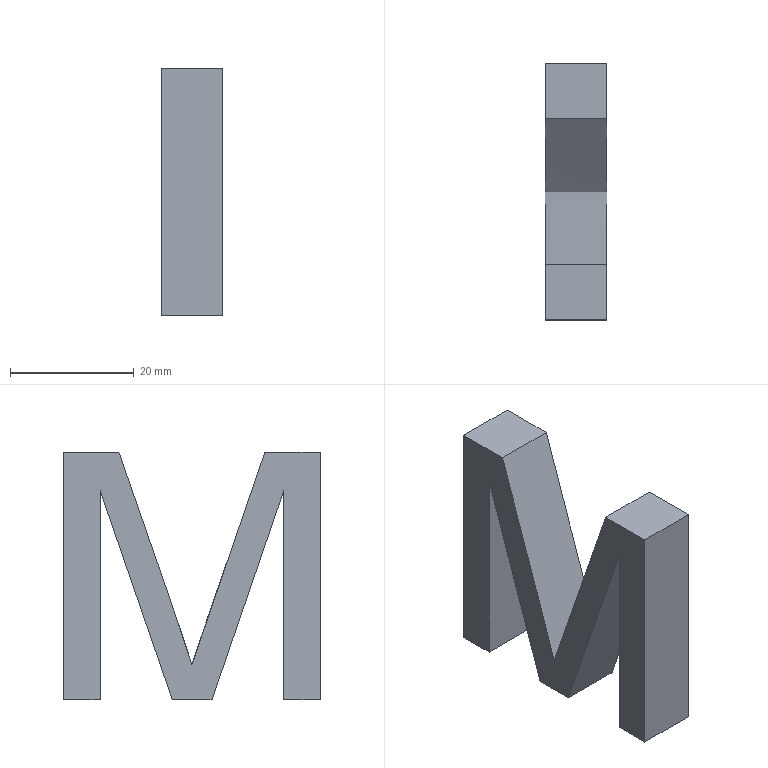Part | NX | features solid 2 | 1 solid | 15 faces | box 10 x 41.407 x 40 mm | volume 8614 mm3 | plane 13 | spline 2
STEP:
#1=CARTESIAN_POINT('',(2250.,-67.941,-590.));
#2=VERTEX_POINT('',#1);
#3=CARTESIAN_POINT('',(2250.,-73.8,-590.));
#4=VERTEX_POINT('',#3);
#5=CARTESIAN_POINT('',(2250.,-67.941,-590.));
#6=CARTESIAN_POINT('',(2250.,-69.894,-590.));
#7=CARTESIAN_POINT('',(2250.,-71.847,-590.));
#8=CARTESIAN_POINT('',(2250.,-73.8,-590.));
#9=B_SPLINE_CURVE_WITH_KNOTS('',3,(#5,#6,#7,#8),.UNSPECIFIED.,.F.,.F.,(4,4),(0.,0.01854),.PIECEWISE_BEZIER_KNOTS.);
#10=EDGE_CURVE('',#2,#4,#9,.T.);
#11=ORIENTED_EDGE('',*,*,#10,.F.);
#12=CARTESIAN_POINT('',(2260.,-67.941,-590.));
#13=VERTEX_POINT('',#12);
#14=CARTESIAN_POINT('',(2260.,-67.941,-590.));
#15=DIRECTION('',(-1.,0.,0.));
#16=VECTOR('',#15,1000.);
#17=LINE('',#14,#16);
#18=EDGE_CURVE('',#13,#2,#17,.T.);
#19=ORIENTED_EDGE('',*,*,#18,.F.);
#20=CARTESIAN_POINT('',(2260.,-73.8,-590.));
#21=VERTEX_POINT('',#20);
#22=CARTESIAN_POINT('',(2260.,-67.941,-590.));
#23=CARTESIAN_POINT('',(2260.,-69.894,-590.));
#24=CARTESIAN_POINT('',(2260.,-71.847,-590.));
#25=CARTESIAN_POINT('',(2260.,-73.8,-590.));
#26=B_SPLINE_CURVE_WITH_KNOTS('',3,(#22,#23,#24,#25),.UNSPECIFIED.,.F.,.F.,(4,4),(0.,0.01854),.PIECEWISE_BEZIER_KNOTS.);
#27=EDGE_CURVE('',#13,#21,#26,.T.);
#28=ORIENTED_EDGE('',*,*,#27,.T.);
#29=CARTESIAN_POINT('',(2260.,-73.8,-590.));
#30=DIRECTION('',(-1.,0.,0.));
#31=VECTOR('',#30,1000.);
#32=LINE('',#29,#31);
#33=EDGE_CURVE('',#21,#4,#32,.T.);
#34=ORIENTED_EDGE('',*,*,#33,.T.);
#35=EDGE_LOOP('',(#11,#19,#28,#34));
#36=FACE_BOUND('',#35,.T.);
#37=CARTESIAN_POINT('',(2260.,-67.941,-590.));
#38=DIRECTION('',(0.,0.,-1.));
#39=DIRECTION('',(-1.,0.,0.));
#40=AXIS2_PLACEMENT_3D('',#37,#38,#39);
#41=PLANE('',#40);
#42=ADVANCED_FACE('',(#36),#41,.T.);
#43=CARTESIAN_POINT('',(2250.,-73.8,-550.));
#44=VERTEX_POINT('',#43);
#45=CARTESIAN_POINT('',(2250.,-73.8,-590.));
#46=CARTESIAN_POINT('',(2250.,-73.8,-576.667));
#47=CARTESIAN_POINT('',(2250.,-73.8,-563.333));
#48=CARTESIAN_POINT('',(2250.,-73.8,-550.));
#49=B_SPLINE_CURVE_WITH_KNOTS('',3,(#45,#46,#47,#48),.UNSPECIFIED.,.F.,.F.,(4,4),(0.01854,0.1451),.PIECEWISE_BEZIER_KNOTS.);
#50=EDGE_CURVE('',#4,#44,#49,.T.);
#51=ORIENTED_EDGE('',*,*,#50,.F.);
#52=ORIENTED_EDGE('',*,*,#33,.F.);
#53=CARTESIAN_POINT('',(2260.,-73.8,-550.));
#54=VERTEX_POINT('',#53);
#55=CARTESIAN_POINT('',(2260.,-73.8,-590.));
#56=CARTESIAN_POINT('',(2260.,-73.8,-576.667));
#57=CARTESIAN_POINT('',(2260.,-73.8,-563.333));
#58=CARTESIAN_POINT('',(2260.,-73.8,-550.));
#59=B_SPLINE_CURVE_WITH_KNOTS('',3,(#55,#56,#57,#58),.UNSPECIFIED.,.F.,.F.,(4,4),(0.01854,0.1451),.PIECEWISE_BEZIER_KNOTS.);
#60=EDGE_CURVE('',#21,#54,#59,.T.);
#61=ORIENTED_EDGE('',*,*,#60,.T.);
#62=CARTESIAN_POINT('',(2260.,-73.8,-550.));
#63=DIRECTION('',(-1.,0.,0.));
#64=VECTOR('',#63,1000.);
#65=LINE('',#62,#64);
#66=EDGE_CURVE('',#54,#44,#65,.T.);
#67=ORIENTED_EDGE('',*,*,#66,.T.);
#68=EDGE_LOOP('',(#51,#52,#61,#67));
#69=FACE_BOUND('',#68,.T.);
#70=CARTESIAN_POINT('',(2260.,-73.8,-590.));
#71=DIRECTION('',(0.,-1.,0.));
#72=DIRECTION('',(1.,0.,0.));
#73=AXIS2_PLACEMENT_3D('',#70,#71,#72);
#74=PLANE('',#73);
#75=ADVANCED_FACE('',(#69),#74,.T.);
#76=CARTESIAN_POINT('',(2250.,-64.852,-550.));
#77=VERTEX_POINT('',#76);
#78=CARTESIAN_POINT('',(2250.,-73.8,-550.));
#79=CARTESIAN_POINT('',(2250.,-70.817,-550.));
#80=CARTESIAN_POINT('',(2250.,-67.834,-550.));
#81=CARTESIAN_POINT('',(2250.,-64.852,-550.));
#82=B_SPLINE_CURVE_WITH_KNOTS('',3,(#78,#79,#80,#81),.UNSPECIFIED.,.F.,.F.,(4,4),(0.1451,0.1734),.PIECEWISE_BEZIER_KNOTS.);
#83=EDGE_CURVE('',#44,#77,#82,.T.);
#84=ORIENTED_EDGE('',*,*,#83,.F.);
#85=ORIENTED_EDGE('',*,*,#66,.F.);
#86=CARTESIAN_POINT('',(2260.,-64.852,-550.));
#87=VERTEX_POINT('',#86);
#88=CARTESIAN_POINT('',(2260.,-73.8,-550.));
#89=CARTESIAN_POINT('',(2260.,-70.817,-550.));
#90=CARTESIAN_POINT('',(2260.,-67.834,-550.));
#91=CARTESIAN_POINT('',(2260.,-64.852,-550.));
#92=B_SPLINE_CURVE_WITH_KNOTS('',3,(#88,#89,#90,#91),.UNSPECIFIED.,.F.,.F.,(4,4),(0.1451,0.1734),.PIECEWISE_BEZIER_KNOTS.);
#93=EDGE_CURVE('',#54,#87,#92,.T.);
#94=ORIENTED_EDGE('',*,*,#93,.T.);
#95=CARTESIAN_POINT('',(2260.,-64.852,-550.));
#96=DIRECTION('',(-1.,0.,0.));
#97=VECTOR('',#96,1000.);
#98=LINE('',#95,#97);
#99=EDGE_CURVE('',#87,#77,#98,.T.);
#100=ORIENTED_EDGE('',*,*,#99,.T.);
#101=EDGE_LOOP('',(#84,#85,#94,#100));
#102=FACE_BOUND('',#101,.T.);
#103=CARTESIAN_POINT('',(2260.,-73.8,-550.));
#104=DIRECTION('',(0.,0.,1.));
#105=DIRECTION('',(1.,0.,0.));
#106=AXIS2_PLACEMENT_3D('',#103,#104,#105);
#107=PLANE('',#106);
#108=ADVANCED_FACE('',(#102),#107,.T.);
#109=CARTESIAN_POINT('',(2250.,-53.089,-584.279));
#110=VERTEX_POINT('',#109);
#111=CARTESIAN_POINT('',(2250.,-64.852,-550.));
#112=CARTESIAN_POINT('',(2250.,-61.593,-559.453));
#113=CARTESIAN_POINT('',(2250.,-58.335,-568.906));
#114=CARTESIAN_POINT('',(2250.,-54.16,-581.021));
#115=CARTESIAN_POINT('',(2250.,-53.502,-582.994));
#116=CARTESIAN_POINT('',(2250.,-53.089,-584.279));
#117=B_SPLINE_CURVE_WITH_KNOTS('',3,(#111,#112,#113,#114,#115,#116),.UNSPECIFIED.,.F.,.F.,(4,2,4),(0.1734,0.2684,0.2951),.UNSPECIFIED.);
#118=EDGE_CURVE('',#77,#110,#117,.T.);
#119=ORIENTED_EDGE('',*,*,#118,.F.);
#120=ORIENTED_EDGE('',*,*,#99,.F.);
#121=CARTESIAN_POINT('',(2260.,-53.089,-584.279));
#122=VERTEX_POINT('',#121);
#123=CARTESIAN_POINT('',(2260.,-64.852,-550.));
#124=CARTESIAN_POINT('',(2260.,-61.593,-559.453));
#125=CARTESIAN_POINT('',(2260.,-58.335,-568.906));
#126=CARTESIAN_POINT('',(2260.,-54.16,-581.021));
#127=CARTESIAN_POINT('',(2260.,-53.502,-582.994));
#128=CARTESIAN_POINT('',(2260.,-53.089,-584.279));
#129=B_SPLINE_CURVE_WITH_KNOTS('',3,(#123,#124,#125,#126,#127,#128),.UNSPECIFIED.,.F.,.F.,(4,2,4),(0.1734,0.2684,0.2951),.UNSPECIFIED.);
#130=EDGE_CURVE('',#87,#122,#129,.T.);
#131=ORIENTED_EDGE('',*,*,#130,.T.);
#132=CARTESIAN_POINT('',(2260.,-53.089,-584.279));
#133=DIRECTION('',(-1.,0.,0.));
#134=VECTOR('',#133,1000.);
#135=LINE('',#132,#134);
#136=EDGE_CURVE('',#122,#110,#135,.T.);
#137=ORIENTED_EDGE('',*,*,#136,.T.);
#138=EDGE_LOOP('',(#119,#120,#131,#137));
#139=FACE_BOUND('',#138,.T.);
#140=CARTESIAN_POINT('',(2260.,-64.852,-550.));
#141=CARTESIAN_POINT('',(2250.,-64.852,-550.));
#142=CARTESIAN_POINT('',(2260.,-63.808,-553.029));
#143=CARTESIAN_POINT('',(2250.,-63.808,-553.029));
#144=CARTESIAN_POINT('',(2260.,-61.72,-559.087));
#145=CARTESIAN_POINT('',(2250.,-61.72,-559.087));
#146=CARTESIAN_POINT('',(2260.,-59.111,-566.656));
#147=CARTESIAN_POINT('',(2250.,-59.111,-566.656));
#148=CARTESIAN_POINT('',(2260.,-57.021,-572.719));
#149=CARTESIAN_POINT('',(2250.,-57.021,-572.719));
#150=CARTESIAN_POINT('',(2260.,-55.721,-576.492));
#151=CARTESIAN_POINT('',(2250.,-55.721,-576.492));
#152=CARTESIAN_POINT('',(2260.,-54.668,-579.546));
#153=CARTESIAN_POINT('',(2250.,-54.668,-579.546));
#154=CARTESIAN_POINT('',(2260.,-53.796,-582.114));
#155=CARTESIAN_POINT('',(2250.,-53.796,-582.114));
#156=CARTESIAN_POINT('',(2260.,-53.324,-583.548));
#157=CARTESIAN_POINT('',(2250.,-53.324,-583.548));
#158=CARTESIAN_POINT('',(2260.,-53.089,-584.279));
#159=CARTESIAN_POINT('',(2250.,-53.089,-584.279));
#160=B_SPLINE_SURFACE_WITH_KNOTS('',3,1,((#140,#141),(#142,#143),(#144,#145),(#146,#147),(#148,#149),(#150,#151),(#152,#153),(#154,#155),(#156,#157),(#158,#159)),.SURF_OF_LINEAR_EXTRUSION.,.F.,.F.,.F.,(4,1,1,1,1,1,1,4),(2,2),(0.1734,0.2039,0.2343,0.2495,0.2647,0.2723,0.2799,0.2951),(0.,1.),.UNSPECIFIED.);
#161=ADVANCED_FACE('',(#139),#160,.T.);
#162=CARTESIAN_POINT('',(2250.,-41.295,-550.));
#163=VERTEX_POINT('',#162);
#164=CARTESIAN_POINT('',(2250.,-53.089,-584.279));
#165=CARTESIAN_POINT('',(2250.,-52.615,-582.841));
#166=CARTESIAN_POINT('',(2250.,-51.911,-580.715));
#167=CARTESIAN_POINT('',(2250.,-47.793,-568.558));
#168=CARTESIAN_POINT('',(2250.,-44.513,-559.29));
#169=CARTESIAN_POINT('',(2250.,-41.295,-550.));
#170=B_SPLINE_CURVE_WITH_KNOTS('',3,(#164,#165,#166,#167,#168,#169),.UNSPECIFIED.,.F.,.F.,(4,2,4),(0.2951,0.317,0.3887),.UNSPECIFIED.);
#171=EDGE_CURVE('',#110,#163,#170,.T.);
#172=ORIENTED_EDGE('',*,*,#171,.F.);
#173=ORIENTED_EDGE('',*,*,#136,.F.);
#174=CARTESIAN_POINT('',(2260.,-41.295,-550.));
#175=VERTEX_POINT('',#174);
#176=CARTESIAN_POINT('',(2260.,-53.089,-584.279));
#177=CARTESIAN_POINT('',(2260.,-52.615,-582.841));
#178=CARTESIAN_POINT('',(2260.,-51.911,-580.715));
#179=CARTESIAN_POINT('',(2260.,-47.793,-568.558));
#180=CARTESIAN_POINT('',(2260.,-44.513,-559.29));
#181=CARTESIAN_POINT('',(2260.,-41.295,-550.));
#182=B_SPLINE_CURVE_WITH_KNOTS('',3,(#176,#177,#178,#179,#180,#181),.UNSPECIFIED.,.F.,.F.,(4,2,4),(0.2951,0.317,0.3887),.UNSPECIFIED.);
#183=EDGE_CURVE('',#122,#175,#182,.T.);
#184=ORIENTED_EDGE('',*,*,#183,.T.);
#185=CARTESIAN_POINT('',(2260.,-41.295,-550.));
#186=DIRECTION('',(-1.,0.,0.));
#187=VECTOR('',#186,1000.);
#188=LINE('',#185,#187);
#189=EDGE_CURVE('',#175,#163,#188,.T.);
#190=ORIENTED_EDGE('',*,*,#189,.T.);
#191=EDGE_LOOP('',(#172,#173,#184,#190));
#192=FACE_BOUND('',#191,.T.);
#193=CARTESIAN_POINT('',(2260.,-53.089,-584.279));
#194=CARTESIAN_POINT('',(2250.,-53.089,-584.279));
#195=CARTESIAN_POINT('',(2260.,-52.835,-583.511));
#196=CARTESIAN_POINT('',(2250.,-52.835,-583.511));
#197=CARTESIAN_POINT('',(2260.,-52.355,-582.059));
#198=CARTESIAN_POINT('',(2250.,-52.355,-582.059));
#199=CARTESIAN_POINT('',(2260.,-51.513,-579.543));
#200=CARTESIAN_POINT('',(2250.,-51.513,-579.543));
#201=CARTESIAN_POINT('',(2260.,-50.499,-576.542));
#202=CARTESIAN_POINT('',(2250.,-50.499,-576.542));
#203=CARTESIAN_POINT('',(2260.,-49.195,-572.727));
#204=CARTESIAN_POINT('',(2250.,-49.195,-572.727));
#205=CARTESIAN_POINT('',(2260.,-47.103,-566.669));
#206=CARTESIAN_POINT('',(2250.,-47.103,-566.669));
#207=CARTESIAN_POINT('',(2260.,-44.459,-559.091));
#208=CARTESIAN_POINT('',(2250.,-44.459,-559.091));
#209=CARTESIAN_POINT('',(2260.,-42.345,-553.032));
#210=CARTESIAN_POINT('',(2250.,-42.345,-553.032));
#211=CARTESIAN_POINT('',(2260.,-41.295,-550.));
#212=CARTESIAN_POINT('',(2250.,-41.295,-550.));
#213=B_SPLINE_SURFACE_WITH_KNOTS('',3,1,((#193,#194),(#195,#196),(#197,#198),(#199,#200),(#201,#202),(#203,#204),(#205,#206),(#207,#208),(#209,#210),(#211,#212)),.SURF_OF_LINEAR_EXTRUSION.,.F.,.F.,.F.,(4,1,1,1,1,1,1,4),(2,2),(0.2951,0.3068,0.3126,0.3185,0.3302,0.3419,0.3653,0.3887),(0.,1.),.UNSPECIFIED.);
#214=ADVANCED_FACE('',(#192),#213,.T.);
#215=CARTESIAN_POINT('',(2250.,-32.393,-550.));
#216=VERTEX_POINT('',#215);
#217=CARTESIAN_POINT('',(2250.,-41.295,-550.));
#218=CARTESIAN_POINT('',(2250.,-38.328,-550.));
#219=CARTESIAN_POINT('',(2250.,-35.36,-550.));
#220=CARTESIAN_POINT('',(2250.,-32.393,-550.));
#221=B_SPLINE_CURVE_WITH_KNOTS('',3,(#217,#218,#219,#220),.UNSPECIFIED.,.F.,.F.,(4,4),(0.3887,0.4159),.PIECEWISE_BEZIER_KNOTS.);
#222=EDGE_CURVE('',#163,#216,#221,.T.);
#223=ORIENTED_EDGE('',*,*,#222,.F.);
#224=ORIENTED_EDGE('',*,*,#189,.F.);
#225=CARTESIAN_POINT('',(2260.,-32.393,-550.));
#226=VERTEX_POINT('',#225);
#227=CARTESIAN_POINT('',(2260.,-41.295,-550.));
#228=CARTESIAN_POINT('',(2260.,-38.328,-550.));
#229=CARTESIAN_POINT('',(2260.,-35.36,-550.));
#230=CARTESIAN_POINT('',(2260.,-32.393,-550.));
#231=B_SPLINE_CURVE_WITH_KNOTS('',3,(#227,#228,#229,#230),.UNSPECIFIED.,.F.,.F.,(4,4),(0.3887,0.4159),.PIECEWISE_BEZIER_KNOTS.);
#232=EDGE_CURVE('',#175,#226,#231,.T.);
#233=ORIENTED_EDGE('',*,*,#232,.T.);
#234=CARTESIAN_POINT('',(2260.,-32.393,-550.));
#235=DIRECTION('',(-1.,0.,0.));
#236=VECTOR('',#235,1000.);
#237=LINE('',#234,#236);
#238=EDGE_CURVE('',#226,#216,#237,.T.);
#239=ORIENTED_EDGE('',*,*,#238,.T.);
#240=EDGE_LOOP('',(#223,#224,#233,#239));
#241=FACE_BOUND('',#240,.T.);
#242=CARTESIAN_POINT('',(2260.,-41.295,-550.));
#243=DIRECTION('',(0.,0.,1.));
#244=DIRECTION('',(1.,0.,0.));
#245=AXIS2_PLACEMENT_3D('',#242,#243,#244);
#246=PLANE('',#245);
#247=ADVANCED_FACE('',(#241),#246,.T.);
#248=CARTESIAN_POINT('',(2250.,-32.393,-590.));
#249=VERTEX_POINT('',#248);
#250=CARTESIAN_POINT('',(2250.,-32.393,-550.));
#251=CARTESIAN_POINT('',(2250.,-32.393,-563.333));
#252=CARTESIAN_POINT('',(2250.,-32.393,-576.667));
#253=CARTESIAN_POINT('',(2250.,-32.393,-590.));
#254=B_SPLINE_CURVE_WITH_KNOTS('',3,(#250,#251,#252,#253),.UNSPECIFIED.,.F.,.F.,(4,4),(0.4159,0.538),.PIECEWISE_BEZIER_KNOTS.);
#255=EDGE_CURVE('',#216,#249,#254,.T.);
#256=ORIENTED_EDGE('',*,*,#255,.F.);
#257=ORIENTED_EDGE('',*,*,#238,.F.);
#258=CARTESIAN_POINT('',(2260.,-32.393,-590.));
#259=VERTEX_POINT('',#258);
#260=CARTESIAN_POINT('',(2260.,-32.393,-550.));
#261=CARTESIAN_POINT('',(2260.,-32.393,-563.333));
#262=CARTESIAN_POINT('',(2260.,-32.393,-576.667));
#263=CARTESIAN_POINT('',(2260.,-32.393,-590.));
#264=B_SPLINE_CURVE_WITH_KNOTS('',3,(#260,#261,#262,#263),.UNSPECIFIED.,.F.,.F.,(4,4),(0.4159,0.538),.PIECEWISE_BEZIER_KNOTS.);
#265=EDGE_CURVE('',#226,#259,#264,.T.);
#266=ORIENTED_EDGE('',*,*,#265,.T.);
#267=CARTESIAN_POINT('',(2260.,-32.393,-590.));
#268=DIRECTION('',(-1.,0.,0.));
#269=VECTOR('',#268,1000.);
#270=LINE('',#267,#269);
#271=EDGE_CURVE('',#259,#249,#270,.T.);
#272=ORIENTED_EDGE('',*,*,#271,.T.);
#273=EDGE_LOOP('',(#256,#257,#266,#272));
#274=FACE_BOUND('',#273,.T.);
#275=CARTESIAN_POINT('',(2260.,-32.393,-550.));
#276=DIRECTION('',(0.,1.,0.));
#277=DIRECTION('',(-1.,0.,0.));
#278=AXIS2_PLACEMENT_3D('',#275,#276,#277);
#279=PLANE('',#278);
#280=ADVANCED_FACE('',(#274),#279,.T.);
#281=CARTESIAN_POINT('',(2250.,-38.236,-590.));
#282=VERTEX_POINT('',#281);
#283=CARTESIAN_POINT('',(2250.,-32.393,-590.));
#284=CARTESIAN_POINT('',(2250.,-34.34,-590.));
#285=CARTESIAN_POINT('',(2250.,-36.288,-590.));
#286=CARTESIAN_POINT('',(2250.,-38.236,-590.));
#287=B_SPLINE_CURVE_WITH_KNOTS('',3,(#283,#284,#285,#286),.UNSPECIFIED.,.F.,.F.,(4,4),(0.538,0.5558),.PIECEWISE_BEZIER_KNOTS.);
#288=EDGE_CURVE('',#249,#282,#287,.T.);
#289=ORIENTED_EDGE('',*,*,#288,.F.);
#290=ORIENTED_EDGE('',*,*,#271,.F.);
#291=CARTESIAN_POINT('',(2260.,-38.236,-590.));
#292=VERTEX_POINT('',#291);
#293=CARTESIAN_POINT('',(2260.,-32.393,-590.));
#294=CARTESIAN_POINT('',(2260.,-34.34,-590.));
#295=CARTESIAN_POINT('',(2260.,-36.288,-590.));
#296=CARTESIAN_POINT('',(2260.,-38.236,-590.));
#297=B_SPLINE_CURVE_WITH_KNOTS('',3,(#293,#294,#295,#296),.UNSPECIFIED.,.F.,.F.,(4,4),(0.538,0.5558),.PIECEWISE_BEZIER_KNOTS.);
#298=EDGE_CURVE('',#259,#292,#297,.T.);
#299=ORIENTED_EDGE('',*,*,#298,.T.);
#300=CARTESIAN_POINT('',(2260.,-38.236,-590.));
#301=DIRECTION('',(-1.,0.,0.));
#302=VECTOR('',#301,1000.);
#303=LINE('',#300,#302);
#304=EDGE_CURVE('',#292,#282,#303,.T.);
#305=ORIENTED_EDGE('',*,*,#304,.T.);
#306=EDGE_LOOP('',(#289,#290,#299,#305));
#307=FACE_BOUND('',#306,.T.);
#308=CARTESIAN_POINT('',(2260.,-32.393,-590.));
#309=DIRECTION('',(0.,0.,-1.));
#310=DIRECTION('',(-1.,0.,0.));
#311=AXIS2_PLACEMENT_3D('',#308,#309,#310);
#312=PLANE('',#311);
#313=ADVANCED_FACE('',(#307),#312,.T.);
#314=CARTESIAN_POINT('',(2250.,-38.236,-556.21));
#315=VERTEX_POINT('',#314);
#316=CARTESIAN_POINT('',(2250.,-38.236,-590.));
#317=CARTESIAN_POINT('',(2250.,-38.236,-578.737));
#318=CARTESIAN_POINT('',(2250.,-38.236,-567.474));
#319=CARTESIAN_POINT('',(2250.,-38.236,-556.21));
#320=B_SPLINE_CURVE_WITH_KNOTS('',3,(#316,#317,#318,#319),.UNSPECIFIED.,.F.,.F.,(4,4),(0.5558,0.659),.PIECEWISE_BEZIER_KNOTS.);
#321=EDGE_CURVE('',#282,#315,#320,.T.);
#322=ORIENTED_EDGE('',*,*,#321,.F.);
#323=ORIENTED_EDGE('',*,*,#304,.F.);
#324=CARTESIAN_POINT('',(2260.,-38.236,-556.21));
#325=VERTEX_POINT('',#324);
#326=CARTESIAN_POINT('',(2260.,-38.236,-590.));
#327=CARTESIAN_POINT('',(2260.,-38.236,-578.737));
#328=CARTESIAN_POINT('',(2260.,-38.236,-567.474));
#329=CARTESIAN_POINT('',(2260.,-38.236,-556.21));
#330=B_SPLINE_CURVE_WITH_KNOTS('',3,(#326,#327,#328,#329),.UNSPECIFIED.,.F.,.F.,(4,4),(0.5558,0.659),.PIECEWISE_BEZIER_KNOTS.);
#331=EDGE_CURVE('',#292,#325,#330,.T.);
#332=ORIENTED_EDGE('',*,*,#331,.T.);
#333=CARTESIAN_POINT('',(2260.,-38.236,-556.21));
#334=DIRECTION('',(-1.,0.,0.));
#335=VECTOR('',#334,1000.);
#336=LINE('',#333,#335);
#337=EDGE_CURVE('',#325,#315,#336,.T.);
#338=ORIENTED_EDGE('',*,*,#337,.T.);
#339=EDGE_LOOP('',(#322,#323,#332,#338));
#340=FACE_BOUND('',#339,.T.);
#341=CARTESIAN_POINT('',(2260.,-38.236,-590.));
#342=DIRECTION('',(0.,-1.,0.));
#343=DIRECTION('',(1.,0.,0.));
#344=AXIS2_PLACEMENT_3D('',#341,#342,#343);
#345=PLANE('',#344);
#346=ADVANCED_FACE('',(#340),#345,.T.);
#347=CARTESIAN_POINT('',(2250.,-49.907,-590.));
#348=VERTEX_POINT('',#347);
#349=CARTESIAN_POINT('',(2250.,-38.236,-556.21));
#350=CARTESIAN_POINT('',(2250.,-42.126,-567.474));
#351=CARTESIAN_POINT('',(2250.,-46.017,-578.737));
#352=CARTESIAN_POINT('',(2250.,-49.907,-590.));
#353=B_SPLINE_CURVE_WITH_KNOTS('',3,(#349,#350,#351,#352),.UNSPECIFIED.,.F.,.F.,(4,4),(0.659,0.7681),.PIECEWISE_BEZIER_KNOTS.);
#354=EDGE_CURVE('',#315,#348,#353,.T.);
#355=ORIENTED_EDGE('',*,*,#354,.F.);
#356=ORIENTED_EDGE('',*,*,#337,.F.);
#357=CARTESIAN_POINT('',(2260.,-49.907,-590.));
#358=VERTEX_POINT('',#357);
#359=CARTESIAN_POINT('',(2260.,-38.236,-556.21));
#360=CARTESIAN_POINT('',(2260.,-42.126,-567.474));
#361=CARTESIAN_POINT('',(2260.,-46.017,-578.737));
#362=CARTESIAN_POINT('',(2260.,-49.907,-590.));
#363=B_SPLINE_CURVE_WITH_KNOTS('',3,(#359,#360,#361,#362),.UNSPECIFIED.,.F.,.F.,(4,4),(0.659,0.7681),.PIECEWISE_BEZIER_KNOTS.);
#364=EDGE_CURVE('',#325,#358,#363,.T.);
#365=ORIENTED_EDGE('',*,*,#364,.T.);
#366=CARTESIAN_POINT('',(2260.,-49.907,-590.));
#367=DIRECTION('',(-1.,0.,0.));
#368=VECTOR('',#367,1000.);
#369=LINE('',#366,#368);
#370=EDGE_CURVE('',#358,#348,#369,.T.);
#371=ORIENTED_EDGE('',*,*,#370,.T.);
#372=EDGE_LOOP('',(#355,#356,#365,#371));
#373=FACE_BOUND('',#372,.T.);
#374=CARTESIAN_POINT('',(2260.,-38.236,-556.21));
#375=DIRECTION('',(0.,0.9452,-0.3265));
#376=DIRECTION('',(0.,0.3265,0.9452));
#377=AXIS2_PLACEMENT_3D('',#374,#375,#376);
#378=PLANE('',#377);
#379=ADVANCED_FACE('',(#373),#378,.T.);
#380=CARTESIAN_POINT('',(2250.,-56.332,-590.));
#381=VERTEX_POINT('',#380);
#382=CARTESIAN_POINT('',(2250.,-49.907,-590.));
#383=CARTESIAN_POINT('',(2250.,-52.049,-590.));
#384=CARTESIAN_POINT('',(2250.,-54.19,-590.));
#385=CARTESIAN_POINT('',(2250.,-56.332,-590.));
#386=B_SPLINE_CURVE_WITH_KNOTS('',3,(#382,#383,#384,#385),.UNSPECIFIED.,.F.,.F.,(4,4),(0.7681,0.7877),.PIECEWISE_BEZIER_KNOTS.);
#387=EDGE_CURVE('',#348,#381,#386,.T.);
#388=ORIENTED_EDGE('',*,*,#387,.F.);
#389=ORIENTED_EDGE('',*,*,#370,.F.);
#390=CARTESIAN_POINT('',(2260.,-56.332,-590.));
#391=VERTEX_POINT('',#390);
#392=CARTESIAN_POINT('',(2260.,-49.907,-590.));
#393=CARTESIAN_POINT('',(2260.,-52.049,-590.));
#394=CARTESIAN_POINT('',(2260.,-54.19,-590.));
#395=CARTESIAN_POINT('',(2260.,-56.332,-590.));
#396=B_SPLINE_CURVE_WITH_KNOTS('',3,(#392,#393,#394,#395),.UNSPECIFIED.,.F.,.F.,(4,4),(0.7681,0.7877),.PIECEWISE_BEZIER_KNOTS.);
#397=EDGE_CURVE('',#358,#391,#396,.T.);
#398=ORIENTED_EDGE('',*,*,#397,.T.);
#399=CARTESIAN_POINT('',(2260.,-56.332,-590.));
#400=DIRECTION('',(-1.,0.,0.));
#401=VECTOR('',#400,1000.);
#402=LINE('',#399,#401);
#403=EDGE_CURVE('',#391,#381,#402,.T.);
#404=ORIENTED_EDGE('',*,*,#403,.T.);
#405=EDGE_LOOP('',(#388,#389,#398,#404));
#406=FACE_BOUND('',#405,.T.);
#407=CARTESIAN_POINT('',(2260.,-49.907,-590.));
#408=DIRECTION('',(0.,0.,-1.));
#409=DIRECTION('',(-1.,0.,0.));
#410=AXIS2_PLACEMENT_3D('',#407,#408,#409);
#411=PLANE('',#410);
#412=ADVANCED_FACE('',(#406),#411,.T.);
#413=CARTESIAN_POINT('',(2250.,-67.941,-556.21));
#414=VERTEX_POINT('',#413);
#415=CARTESIAN_POINT('',(2250.,-56.332,-590.));
#416=CARTESIAN_POINT('',(2250.,-60.202,-578.737));
#417=CARTESIAN_POINT('',(2250.,-64.072,-567.474));
#418=CARTESIAN_POINT('',(2250.,-67.941,-556.21));
#419=B_SPLINE_CURVE_WITH_KNOTS('',3,(#415,#416,#417,#418),.UNSPECIFIED.,.F.,.F.,(4,4),(0.7877,0.8968),.PIECEWISE_BEZIER_KNOTS.);
#420=EDGE_CURVE('',#381,#414,#419,.T.);
#421=ORIENTED_EDGE('',*,*,#420,.F.);
#422=ORIENTED_EDGE('',*,*,#403,.F.);
#423=CARTESIAN_POINT('',(2260.,-67.941,-556.21));
#424=VERTEX_POINT('',#423);
#425=CARTESIAN_POINT('',(2260.,-56.332,-590.));
#426=CARTESIAN_POINT('',(2260.,-60.202,-578.737));
#427=CARTESIAN_POINT('',(2260.,-64.072,-567.474));
#428=CARTESIAN_POINT('',(2260.,-67.941,-556.21));
#429=B_SPLINE_CURVE_WITH_KNOTS('',3,(#425,#426,#427,#428),.UNSPECIFIED.,.F.,.F.,(4,4),(0.7877,0.8968),.PIECEWISE_BEZIER_KNOTS.);
#430=EDGE_CURVE('',#391,#424,#429,.T.);
#431=ORIENTED_EDGE('',*,*,#430,.T.);
#432=CARTESIAN_POINT('',(2260.,-67.941,-556.21));
#433=DIRECTION('',(-1.,0.,0.));
#434=VECTOR('',#433,1000.);
#435=LINE('',#432,#434);
#436=EDGE_CURVE('',#424,#414,#435,.T.);
#437=ORIENTED_EDGE('',*,*,#436,.T.);
#438=EDGE_LOOP('',(#421,#422,#431,#437));
#439=FACE_BOUND('',#438,.T.);
#440=CARTESIAN_POINT('',(2260.,-56.332,-590.));
#441=DIRECTION('',(0.,-0.9457,-0.3249));
#442=DIRECTION('',(0.,0.3249,-0.9457));
#443=AXIS2_PLACEMENT_3D('',#440,#441,#442);
#444=PLANE('',#443);
#445=ADVANCED_FACE('',(#439),#444,.T.);
#446=CARTESIAN_POINT('',(2250.,-67.941,-556.21));
#447=CARTESIAN_POINT('',(2250.,-67.941,-567.474));
#448=CARTESIAN_POINT('',(2250.,-67.941,-578.737));
#449=CARTESIAN_POINT('',(2250.,-67.941,-590.));
#450=B_SPLINE_CURVE_WITH_KNOTS('',3,(#446,#447,#448,#449),.UNSPECIFIED.,.F.,.F.,(4,4),(0.8968,1.),.PIECEWISE_BEZIER_KNOTS.);
#451=EDGE_CURVE('',#414,#2,#450,.T.);
#452=ORIENTED_EDGE('',*,*,#451,.F.);
#453=ORIENTED_EDGE('',*,*,#436,.F.);
#454=CARTESIAN_POINT('',(2260.,-67.941,-556.21));
#455=CARTESIAN_POINT('',(2260.,-67.941,-567.474));
#456=CARTESIAN_POINT('',(2260.,-67.941,-578.737));
#457=CARTESIAN_POINT('',(2260.,-67.941,-590.));
#458=B_SPLINE_CURVE_WITH_KNOTS('',3,(#454,#455,#456,#457),.UNSPECIFIED.,.F.,.F.,(4,4),(0.8968,1.),.PIECEWISE_BEZIER_KNOTS.);
#459=EDGE_CURVE('',#424,#13,#458,.T.);
#460=ORIENTED_EDGE('',*,*,#459,.T.);
#461=ORIENTED_EDGE('',*,*,#18,.T.);
#462=EDGE_LOOP('',(#452,#453,#460,#461));
#463=FACE_BOUND('',#462,.T.);
#464=CARTESIAN_POINT('',(2260.,-67.941,-556.21));
#465=DIRECTION('',(0.,1.,0.));
#466=DIRECTION('',(-1.,0.,0.));
#467=AXIS2_PLACEMENT_3D('',#464,#465,#466);
#468=PLANE('',#467);
#469=ADVANCED_FACE('',(#463),#468,.T.);
#470=ORIENTED_EDGE('',*,*,#27,.F.);
#471=ORIENTED_EDGE('',*,*,#459,.F.);
#472=ORIENTED_EDGE('',*,*,#430,.F.);
#473=ORIENTED_EDGE('',*,*,#397,.F.);
#474=ORIENTED_EDGE('',*,*,#364,.F.);
#475=ORIENTED_EDGE('',*,*,#331,.F.);
#476=ORIENTED_EDGE('',*,*,#298,.F.);
#477=ORIENTED_EDGE('',*,*,#265,.F.);
#478=ORIENTED_EDGE('',*,*,#232,.F.);
#479=ORIENTED_EDGE('',*,*,#183,.F.);
#480=ORIENTED_EDGE('',*,*,#130,.F.);
#481=ORIENTED_EDGE('',*,*,#93,.F.);
#482=ORIENTED_EDGE('',*,*,#60,.F.);
#483=EDGE_LOOP('',(#470,#471,#472,#473,#474,#475,#476,#477,#478,#479,#480,#481,#482));
#484=FACE_BOUND('',#483,.T.);
#485=CARTESIAN_POINT('',(2260.,-58.588,-568.172));
#486=DIRECTION('',(1.,0.,0.));
#487=DIRECTION('',(0.,1.,0.));
#488=AXIS2_PLACEMENT_3D('',#485,#486,#487);
#489=PLANE('',#488);
#490=ADVANCED_FACE('',(#484),#489,.T.);
#491=ORIENTED_EDGE('',*,*,#10,.T.);
#492=ORIENTED_EDGE('',*,*,#50,.T.);
#493=ORIENTED_EDGE('',*,*,#83,.T.);
#494=ORIENTED_EDGE('',*,*,#118,.T.);
#495=ORIENTED_EDGE('',*,*,#171,.T.);
#496=ORIENTED_EDGE('',*,*,#222,.T.);
#497=ORIENTED_EDGE('',*,*,#255,.T.);
#498=ORIENTED_EDGE('',*,*,#288,.T.);
#499=ORIENTED_EDGE('',*,*,#321,.T.);
#500=ORIENTED_EDGE('',*,*,#354,.T.);
#501=ORIENTED_EDGE('',*,*,#387,.T.);
#502=ORIENTED_EDGE('',*,*,#420,.T.);
#503=ORIENTED_EDGE('',*,*,#451,.T.);
#504=EDGE_LOOP('',(#491,#492,#493,#494,#495,#496,#497,#498,#499,#500,#501,#502,#503));
#505=FACE_BOUND('',#504,.T.);
#506=CARTESIAN_POINT('',(2250.,-58.588,-568.172));
#507=DIRECTION('',(1.,0.,0.));
#508=DIRECTION('',(0.,1.,0.));
#509=AXIS2_PLACEMENT_3D('',#506,#507,#508);
#510=PLANE('',#509);
#511=ADVANCED_FACE('',(#505),#510,.F.);
#512=CLOSED_SHELL('',(#42,#75,#108,#161,#214,#247,#280,#313,#346,#379,#412,#445,#469,#490,#511));
#513=MANIFOLD_SOLID_BREP('',#512);
#514=(LENGTH_UNIT()NAMED_UNIT(*)SI_UNIT(.MILLI.,.METRE.));
#515=UNCERTAINTY_MEASURE_WITH_UNIT(LENGTH_MEASURE(0.0508),#514,'','');
#516=(NAMED_UNIT(*)PLANE_ANGLE_UNIT()SI_UNIT($,.RADIAN.));
#517=(NAMED_UNIT(*)SI_UNIT($,.STERADIAN.)SOLID_ANGLE_UNIT());
#518=(GEOMETRIC_REPRESENTATION_CONTEXT(3)GLOBAL_UNCERTAINTY_ASSIGNED_CONTEXT((#515))GLOBAL_UNIT_ASSIGNED_CONTEXT((#514,#516,#517))REPRESENTATION_CONTEXT('',''));
#519=ADVANCED_BREP_SHAPE_REPRESENTATION('',(#513),#518);